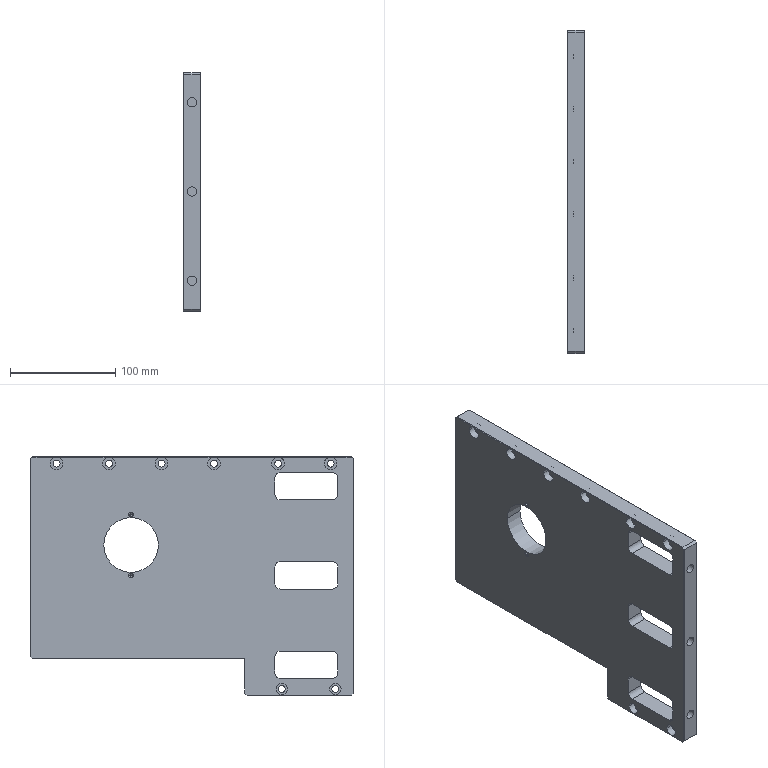Part | NX | 1 solid | 142 faces | box 17 x 308 x 227 mm | volume 939119 mm3 | cylinder 70 | plane 40 | cone 32 | commonest cylinder face diameters 6.6 x16 10 x12 12 x12 3.3 x10 4.2 x6 9 x6